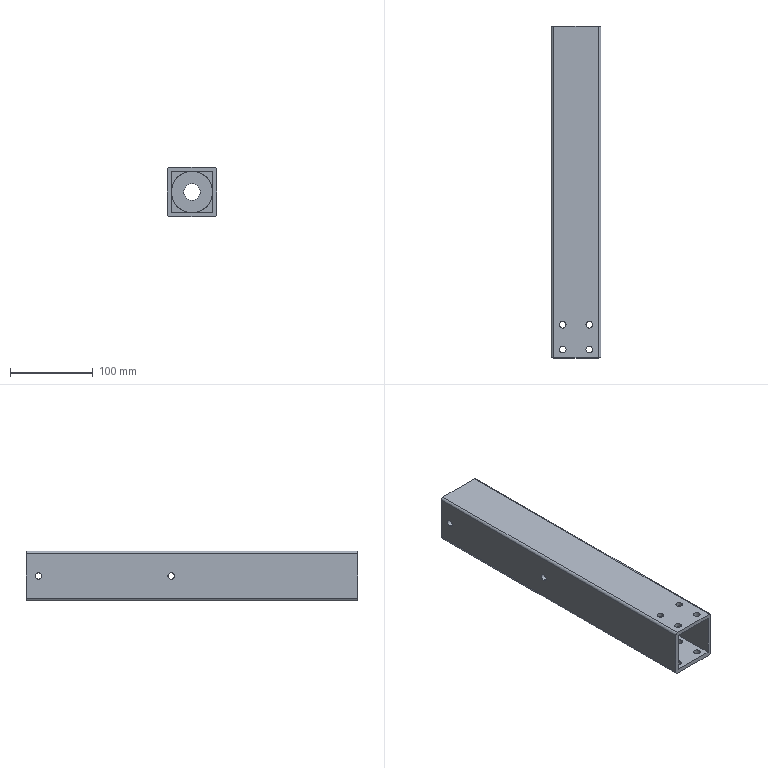Part | SolidWorks | features ICE 9, Fillet 2, Extrusion 1 | 1 solid | 71 faces | box 60 x 400 x 60 mm | volume 650447 mm3 | cylinder 46 | plane 25 | commonest cylinder face diameters 8 x24 5 x8 6 x8 20 x2 40 x2 50 x2